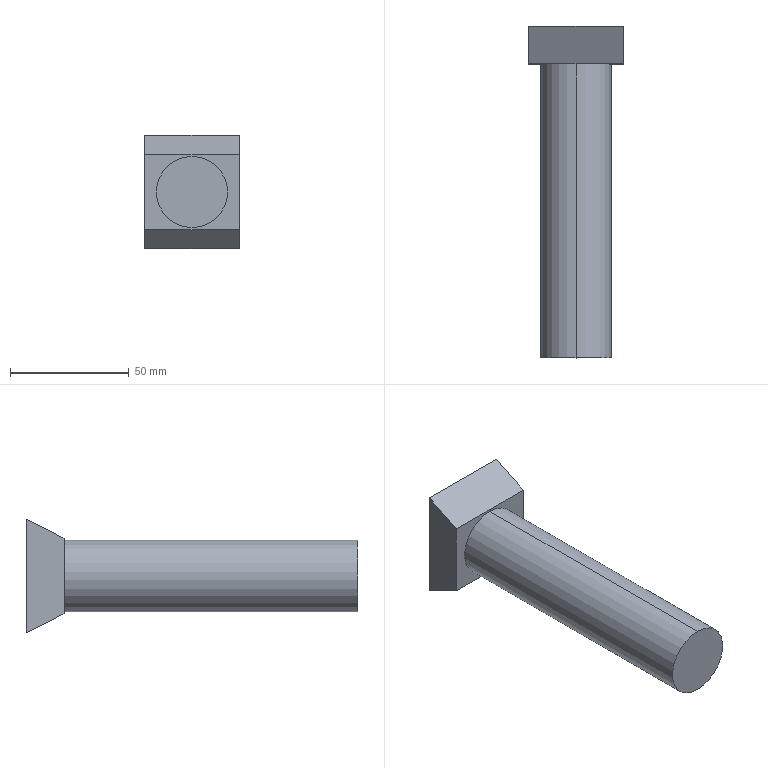Part | SolidWorks | features ICE 2, Extrusion 1 | 1 solid | 9 faces | box 40 x 140 x 48 mm | volume 113250 mm3 | plane 7 | cylinder 2 | commonest cylinder face diameters 30 x2
STEP:
#1=CARTESIAN_POINT('',(0.,-132.,-15.));
#2=VERTEX_POINT('',#1);
#3=CARTESIAN_POINT('',(0.,-132.,15.));
#4=VERTEX_POINT('',#3);
#5=CARTESIAN_POINT('',(0.,-132.,0.));
#6=DIRECTION('',(0.,-1.,0.));
#7=DIRECTION('',(0.,0.,-1.));
#8=AXIS2_PLACEMENT_3D('',#5,#6,#7);
#9=CIRCLE('',#8,15.);
#10=EDGE_CURVE('',#2,#4,#9,.T.);
#11=ORIENTED_EDGE('',*,*,#10,.F.);
#12=CARTESIAN_POINT('',(0.,-8.,-15.));
#13=VERTEX_POINT('',#12);
#14=CARTESIAN_POINT('',(0.,-132.,-15.));
#15=DIRECTION('',(0.,1.,0.));
#16=VECTOR('',#15,1000.);
#17=LINE('',#14,#16);
#18=EDGE_CURVE('',#2,#13,#17,.T.);
#19=ORIENTED_EDGE('',*,*,#18,.T.);
#20=CARTESIAN_POINT('',(0.,-8.,15.));
#21=VERTEX_POINT('',#20);
#22=CARTESIAN_POINT('',(0.,-8.,0.));
#23=DIRECTION('',(0.,-1.,0.));
#24=DIRECTION('',(0.,0.,1.));
#25=AXIS2_PLACEMENT_3D('',#22,#23,#24);
#26=CIRCLE('',#25,15.);
#27=EDGE_CURVE('',#13,#21,#26,.T.);
#28=ORIENTED_EDGE('',*,*,#27,.T.);
#29=CARTESIAN_POINT('',(0.,-132.,15.));
#30=DIRECTION('',(0.,1.,0.));
#31=VECTOR('',#30,1000.);
#32=LINE('',#29,#31);
#33=EDGE_CURVE('',#4,#21,#32,.T.);
#34=ORIENTED_EDGE('',*,*,#33,.F.);
#35=EDGE_LOOP('',(#11,#19,#28,#34));
#36=FACE_OUTER_BOUND('',#35,.T.);
#37=CARTESIAN_POINT('',(0.,-132.,0.));
#38=DIRECTION('',(0.,1.,0.));
#39=DIRECTION('',(0.,0.,1.));
#40=AXIS2_PLACEMENT_3D('',#37,#38,#39);
#41=CYLINDRICAL_SURFACE('',#40,15.);
#42=ADVANCED_FACE('',(#36),#41,.T.);
#43=CARTESIAN_POINT('',(0.,-8.,0.));
#44=DIRECTION('',(0.,-1.,0.));
#45=DIRECTION('',(0.,0.,1.));
#46=AXIS2_PLACEMENT_3D('',#43,#44,#45);
#47=CIRCLE('',#46,15.);
#48=EDGE_CURVE('',#21,#13,#47,.T.);
#49=ORIENTED_EDGE('',*,*,#48,.F.);
#50=ORIENTED_EDGE('',*,*,#27,.F.);
#51=EDGE_LOOP('',(#49,#50));
#52=FACE_BOUND('',#51,.T.);
#53=CARTESIAN_POINT('',(-20.,-8.,16.));
#54=VERTEX_POINT('',#53);
#55=CARTESIAN_POINT('',(-20.,-8.,-16.));
#56=VERTEX_POINT('',#55);
#57=CARTESIAN_POINT('',(-20.,-8.,-24.));
#58=DIRECTION('',(0.,0.,-1.));
#59=VECTOR('',#58,1000.);
#60=LINE('',#57,#59);
#61=EDGE_CURVE('',#54,#56,#60,.T.);
#62=ORIENTED_EDGE('',*,*,#61,.T.);
#63=CARTESIAN_POINT('',(20.,-8.,-16.));
#64=VERTEX_POINT('',#63);
#65=CARTESIAN_POINT('',(-20.,-8.,-16.));
#66=DIRECTION('',(1.,0.,0.));
#67=VECTOR('',#66,1000.);
#68=LINE('',#65,#67);
#69=EDGE_CURVE('',#56,#64,#68,.T.);
#70=ORIENTED_EDGE('',*,*,#69,.T.);
#71=CARTESIAN_POINT('',(20.,-8.,16.));
#72=VERTEX_POINT('',#71);
#73=CARTESIAN_POINT('',(20.,-8.,-24.));
#74=DIRECTION('',(0.,0.,-1.));
#75=VECTOR('',#74,1000.);
#76=LINE('',#73,#75);
#77=EDGE_CURVE('',#72,#64,#76,.T.);
#78=ORIENTED_EDGE('',*,*,#77,.F.);
#79=CARTESIAN_POINT('',(-20.,-8.,16.));
#80=DIRECTION('',(1.,0.,0.));
#81=VECTOR('',#80,1000.);
#82=LINE('',#79,#81);
#83=EDGE_CURVE('',#54,#72,#82,.T.);
#84=ORIENTED_EDGE('',*,*,#83,.F.);
#85=EDGE_LOOP('',(#62,#70,#78,#84));
#86=FACE_OUTER_BOUND('',#85,.T.);
#87=CARTESIAN_POINT('',(20.,-8.,-24.));
#88=DIRECTION('',(0.,1.,0.));
#89=DIRECTION('',(0.,0.,1.));
#90=AXIS2_PLACEMENT_3D('',#87,#88,#89);
#91=PLANE('',#90);
#92=ADVANCED_FACE('',(#52,#86),#91,.F.);
#93=CARTESIAN_POINT('',(-20.,8.,-24.));
#94=VERTEX_POINT('',#93);
#95=CARTESIAN_POINT('',(-20.,8.,24.));
#96=VERTEX_POINT('',#95);
#97=CARTESIAN_POINT('',(-20.,8.,-24.));
#98=DIRECTION('',(0.,0.,1.));
#99=VECTOR('',#98,1000.);
#100=LINE('',#97,#99);
#101=EDGE_CURVE('',#94,#96,#100,.T.);
#102=ORIENTED_EDGE('',*,*,#101,.T.);
#103=CARTESIAN_POINT('',(20.,8.,24.));
#104=VERTEX_POINT('',#103);
#105=CARTESIAN_POINT('',(20.,8.,24.));
#106=DIRECTION('',(-1.,0.,0.));
#107=VECTOR('',#106,1000.);
#108=LINE('',#105,#107);
#109=EDGE_CURVE('',#104,#96,#108,.T.);
#110=ORIENTED_EDGE('',*,*,#109,.F.);
#111=CARTESIAN_POINT('',(20.,8.,-24.));
#112=VERTEX_POINT('',#111);
#113=CARTESIAN_POINT('',(20.,8.,-24.));
#114=DIRECTION('',(0.,0.,1.));
#115=VECTOR('',#114,1000.);
#116=LINE('',#113,#115);
#117=EDGE_CURVE('',#112,#104,#116,.T.);
#118=ORIENTED_EDGE('',*,*,#117,.F.);
#119=CARTESIAN_POINT('',(20.,8.,-24.));
#120=DIRECTION('',(-1.,0.,0.));
#121=VECTOR('',#120,1000.);
#122=LINE('',#119,#121);
#123=EDGE_CURVE('',#112,#94,#122,.T.);
#124=ORIENTED_EDGE('',*,*,#123,.T.);
#125=EDGE_LOOP('',(#102,#110,#118,#124));
#126=FACE_OUTER_BOUND('',#125,.T.);
#127=CARTESIAN_POINT('',(20.,8.,-24.));
#128=DIRECTION('',(0.,-1.,0.));
#129=DIRECTION('',(0.,0.,-1.));
#130=AXIS2_PLACEMENT_3D('',#127,#128,#129);
#131=PLANE('',#130);
#132=ADVANCED_FACE('',(#126),#131,.F.);
#133=CARTESIAN_POINT('',(20.,-8.,-16.));
#134=DIRECTION('',(0.,-0.8944,0.4472));
#135=VECTOR('',#134,1000.);
#136=LINE('',#133,#135);
#137=EDGE_CURVE('',#112,#64,#136,.T.);
#138=ORIENTED_EDGE('',*,*,#137,.F.);
#139=ORIENTED_EDGE('',*,*,#117,.T.);
#140=CARTESIAN_POINT('',(20.,8.,24.));
#141=DIRECTION('',(0.,0.8944,0.4472));
#142=VECTOR('',#141,1000.);
#143=LINE('',#140,#142);
#144=EDGE_CURVE('',#72,#104,#143,.T.);
#145=ORIENTED_EDGE('',*,*,#144,.F.);
#146=ORIENTED_EDGE('',*,*,#77,.T.);
#147=EDGE_LOOP('',(#138,#139,#145,#146));
#148=FACE_OUTER_BOUND('',#147,.T.);
#149=CARTESIAN_POINT('',(20.,0.,0.));
#150=DIRECTION('',(1.,0.,0.));
#151=DIRECTION('',(0.,0.,-1.));
#152=AXIS2_PLACEMENT_3D('',#149,#150,#151);
#153=PLANE('',#152);
#154=ADVANCED_FACE('',(#148),#153,.T.);
#155=ORIENTED_EDGE('',*,*,#101,.F.);
#156=CARTESIAN_POINT('',(-20.,-8.,-16.));
#157=DIRECTION('',(0.,-0.8944,0.4472));
#158=VECTOR('',#157,1000.);
#159=LINE('',#156,#158);
#160=EDGE_CURVE('',#94,#56,#159,.T.);
#161=ORIENTED_EDGE('',*,*,#160,.T.);
#162=ORIENTED_EDGE('',*,*,#61,.F.);
#163=CARTESIAN_POINT('',(-20.,8.,24.));
#164=DIRECTION('',(0.,0.8944,0.4472));
#165=VECTOR('',#164,1000.);
#166=LINE('',#163,#165);
#167=EDGE_CURVE('',#54,#96,#166,.T.);
#168=ORIENTED_EDGE('',*,*,#167,.T.);
#169=EDGE_LOOP('',(#155,#161,#162,#168));
#170=FACE_OUTER_BOUND('',#169,.T.);
#171=CARTESIAN_POINT('',(-20.,0.,0.));
#172=DIRECTION('',(1.,0.,0.));
#173=DIRECTION('',(0.,0.,-1.));
#174=AXIS2_PLACEMENT_3D('',#171,#172,#173);
#175=PLANE('',#174);
#176=ADVANCED_FACE('',(#170),#175,.F.);
#177=ORIENTED_EDGE('',*,*,#109,.T.);
#178=ORIENTED_EDGE('',*,*,#167,.F.);
#179=ORIENTED_EDGE('',*,*,#83,.T.);
#180=ORIENTED_EDGE('',*,*,#144,.T.);
#181=EDGE_LOOP('',(#177,#178,#179,#180));
#182=FACE_OUTER_BOUND('',#181,.T.);
#183=CARTESIAN_POINT('',(-20.,8.,24.));
#184=DIRECTION('',(0.,0.4472,-0.8944));
#185=DIRECTION('',(0.,0.8944,0.4472));
#186=AXIS2_PLACEMENT_3D('',#183,#184,#185);
#187=PLANE('',#186);
#188=ADVANCED_FACE('',(#182),#187,.F.);
#189=ORIENTED_EDGE('',*,*,#69,.F.);
#190=ORIENTED_EDGE('',*,*,#160,.F.);
#191=ORIENTED_EDGE('',*,*,#123,.F.);
#192=ORIENTED_EDGE('',*,*,#137,.T.);
#193=EDGE_LOOP('',(#189,#190,#191,#192));
#194=FACE_OUTER_BOUND('',#193,.T.);
#195=CARTESIAN_POINT('',(-20.,-8.,-16.));
#196=DIRECTION('',(0.,0.4472,0.8944));
#197=DIRECTION('',(0.,-0.8944,0.4472));
#198=AXIS2_PLACEMENT_3D('',#195,#196,#197);
#199=PLANE('',#198);
#200=ADVANCED_FACE('',(#194),#199,.F.);
#201=ORIENTED_EDGE('',*,*,#18,.F.);
#202=CARTESIAN_POINT('',(0.,-132.,0.));
#203=DIRECTION('',(0.,-1.,0.));
#204=DIRECTION('',(0.,0.,-1.));
#205=AXIS2_PLACEMENT_3D('',#202,#203,#204);
#206=CIRCLE('',#205,15.);
#207=EDGE_CURVE('',#4,#2,#206,.T.);
#208=ORIENTED_EDGE('',*,*,#207,.F.);
#209=ORIENTED_EDGE('',*,*,#33,.T.);
#210=ORIENTED_EDGE('',*,*,#48,.T.);
#211=EDGE_LOOP('',(#201,#208,#209,#210));
#212=FACE_OUTER_BOUND('',#211,.T.);
#213=CARTESIAN_POINT('',(0.,-132.,0.));
#214=DIRECTION('',(0.,1.,0.));
#215=DIRECTION('',(0.,0.,1.));
#216=AXIS2_PLACEMENT_3D('',#213,#214,#215);
#217=CYLINDRICAL_SURFACE('',#216,15.);
#218=ADVANCED_FACE('',(#212),#217,.T.);
#219=ORIENTED_EDGE('',*,*,#207,.T.);
#220=ORIENTED_EDGE('',*,*,#10,.T.);
#221=EDGE_LOOP('',(#219,#220));
#222=FACE_OUTER_BOUND('',#221,.T.);
#223=CARTESIAN_POINT('',(0.,-132.,0.));
#224=DIRECTION('',(0.,-1.,0.));
#225=DIRECTION('',(0.,0.,-1.));
#226=AXIS2_PLACEMENT_3D('',#223,#224,#225);
#227=PLANE('',#226);
#228=ADVANCED_FACE('',(#222),#227,.T.);
#229=CLOSED_SHELL('',(#42,#92,#132,#154,#176,#188,#200,#218,#228));
#230=MANIFOLD_SOLID_BREP('',#229);
#231=CARTESIAN_POINT('',(0.,0.,0.));
#232=DIRECTION('',(0.,0.,1.));
#233=DIRECTION('',(1.,0.,0.));
#234=AXIS2_PLACEMENT_3D('',#231,#232,#233);
#235=(LENGTH_UNIT()NAMED_UNIT(*)SI_UNIT(.MILLI.,.METRE.));
#236=UNCERTAINTY_MEASURE_WITH_UNIT(LENGTH_MEASURE(0.00001),#235,'','');
#237=(NAMED_UNIT(*)PLANE_ANGLE_UNIT()SI_UNIT($,.RADIAN.));
#238=(NAMED_UNIT(*)SI_UNIT($,.STERADIAN.)SOLID_ANGLE_UNIT());
#239=(GEOMETRIC_REPRESENTATION_CONTEXT(3)GLOBAL_UNCERTAINTY_ASSIGNED_CONTEXT((#236))GLOBAL_UNIT_ASSIGNED_CONTEXT((#235,#237,#238))REPRESENTATION_CONTEXT('',''));
#240=ADVANCED_BREP_SHAPE_REPRESENTATION('',(#230,#234),#239);